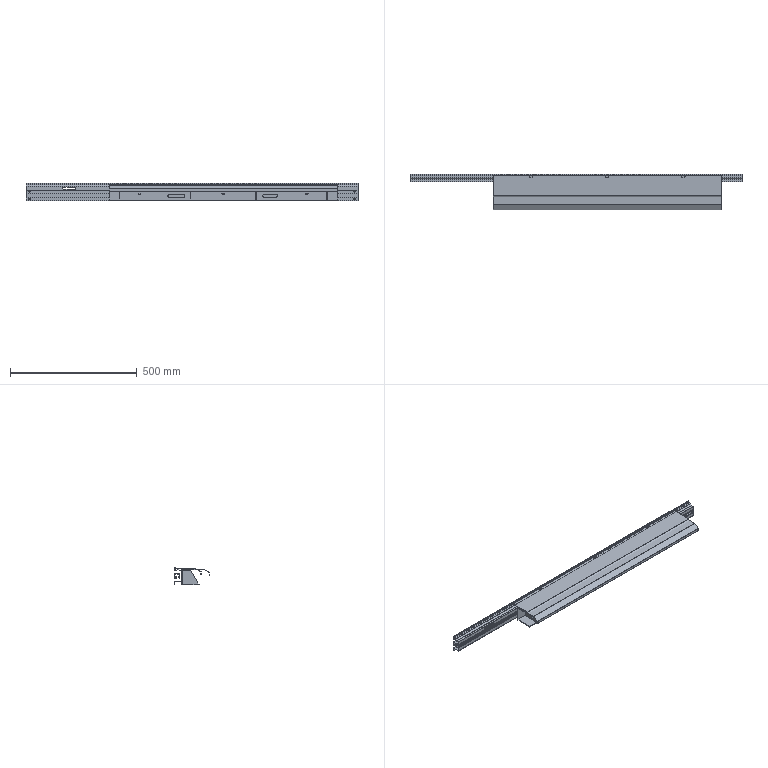Part | SolidWorks | 8 solids | 293 faces | box 1310 x 141.151 x 70 mm | volume 1112125 mm3 | plane 192 | cylinder 101 | commonest cylinder face diameters 10 x21 6 x20 7 x18 9 x12 3 x11 2 x9